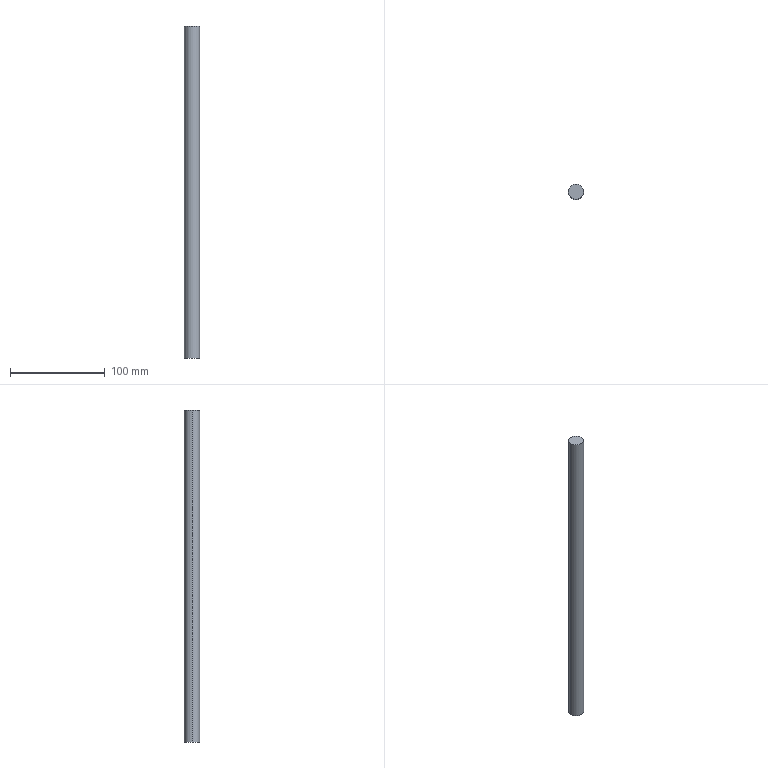Part | SolidWorks | features Extrusion 1 | 1 solid | 4 faces | box 16 x 16 x 350 mm | volume 70372 mm3 | cylinder 2 | plane 2 | commonest cylinder face diameters 16 x2
STEP:
#1=CARTESIAN_POINT('',(8.,0.,350.));
#2=VERTEX_POINT('',#1);
#3=CARTESIAN_POINT('',(-8.,0.,350.));
#4=VERTEX_POINT('',#3);
#5=CARTESIAN_POINT('',(0.,0.,350.));
#6=DIRECTION('',(0.,0.,1.));
#7=DIRECTION('',(1.,0.,0.));
#8=AXIS2_PLACEMENT_3D('',#5,#6,#7);
#9=CIRCLE('',#8,8.);
#10=EDGE_CURVE('',#2,#4,#9,.T.);
#11=ORIENTED_EDGE('',*,*,#10,.F.);
#12=CARTESIAN_POINT('',(8.,0.,0.));
#13=VERTEX_POINT('',#12);
#14=CARTESIAN_POINT('',(8.,0.,350.));
#15=DIRECTION('',(0.,0.,-1.));
#16=VECTOR('',#15,1000.);
#17=LINE('',#14,#16);
#18=EDGE_CURVE('',#2,#13,#17,.T.);
#19=ORIENTED_EDGE('',*,*,#18,.T.);
#20=CARTESIAN_POINT('',(-8.,0.,0.));
#21=VERTEX_POINT('',#20);
#22=CARTESIAN_POINT('',(0.,0.,0.));
#23=DIRECTION('',(0.,0.,1.));
#24=DIRECTION('',(1.,0.,0.));
#25=AXIS2_PLACEMENT_3D('',#22,#23,#24);
#26=CIRCLE('',#25,8.);
#27=EDGE_CURVE('',#13,#21,#26,.T.);
#28=ORIENTED_EDGE('',*,*,#27,.T.);
#29=CARTESIAN_POINT('',(-8.,0.,350.));
#30=DIRECTION('',(0.,0.,-1.));
#31=VECTOR('',#30,1000.);
#32=LINE('',#29,#31);
#33=EDGE_CURVE('',#4,#21,#32,.T.);
#34=ORIENTED_EDGE('',*,*,#33,.F.);
#35=EDGE_LOOP('',(#11,#19,#28,#34));
#36=FACE_OUTER_BOUND('',#35,.T.);
#37=CARTESIAN_POINT('',(0.,0.,350.));
#38=DIRECTION('',(0.,0.,-1.));
#39=DIRECTION('',(-1.,0.,0.));
#40=AXIS2_PLACEMENT_3D('',#37,#38,#39);
#41=CYLINDRICAL_SURFACE('',#40,8.);
#42=ADVANCED_FACE('',(#36),#41,.T.);
#43=ORIENTED_EDGE('',*,*,#18,.F.);
#44=CARTESIAN_POINT('',(0.,0.,350.));
#45=DIRECTION('',(0.,0.,1.));
#46=DIRECTION('',(1.,0.,0.));
#47=AXIS2_PLACEMENT_3D('',#44,#45,#46);
#48=CIRCLE('',#47,8.);
#49=EDGE_CURVE('',#4,#2,#48,.T.);
#50=ORIENTED_EDGE('',*,*,#49,.F.);
#51=ORIENTED_EDGE('',*,*,#33,.T.);
#52=CARTESIAN_POINT('',(0.,0.,0.));
#53=DIRECTION('',(0.,0.,1.));
#54=DIRECTION('',(1.,0.,0.));
#55=AXIS2_PLACEMENT_3D('',#52,#53,#54);
#56=CIRCLE('',#55,8.);
#57=EDGE_CURVE('',#21,#13,#56,.T.);
#58=ORIENTED_EDGE('',*,*,#57,.T.);
#59=EDGE_LOOP('',(#43,#50,#51,#58));
#60=FACE_OUTER_BOUND('',#59,.T.);
#61=CARTESIAN_POINT('',(0.,0.,350.));
#62=DIRECTION('',(0.,0.,-1.));
#63=DIRECTION('',(-1.,0.,0.));
#64=AXIS2_PLACEMENT_3D('',#61,#62,#63);
#65=CYLINDRICAL_SURFACE('',#64,8.);
#66=ADVANCED_FACE('',(#60),#65,.T.);
#67=ORIENTED_EDGE('',*,*,#49,.T.);
#68=ORIENTED_EDGE('',*,*,#10,.T.);
#69=EDGE_LOOP('',(#67,#68));
#70=FACE_OUTER_BOUND('',#69,.T.);
#71=CARTESIAN_POINT('',(0.,0.,350.));
#72=DIRECTION('',(0.,0.,1.));
#73=DIRECTION('',(1.,0.,0.));
#74=AXIS2_PLACEMENT_3D('',#71,#72,#73);
#75=PLANE('',#74);
#76=ADVANCED_FACE('',(#70),#75,.T.);
#77=ORIENTED_EDGE('',*,*,#57,.F.);
#78=ORIENTED_EDGE('',*,*,#27,.F.);
#79=EDGE_LOOP('',(#77,#78));
#80=FACE_OUTER_BOUND('',#79,.T.);
#81=CARTESIAN_POINT('',(0.,0.,0.));
#82=DIRECTION('',(0.,0.,1.));
#83=DIRECTION('',(1.,0.,0.));
#84=AXIS2_PLACEMENT_3D('',#81,#82,#83);
#85=PLANE('',#84);
#86=ADVANCED_FACE('',(#80),#85,.F.);
#87=CLOSED_SHELL('',(#42,#66,#76,#86));
#88=MANIFOLD_SOLID_BREP('',#87);
#89=CARTESIAN_POINT('',(0.,0.,0.));
#90=DIRECTION('',(0.,0.,1.));
#91=DIRECTION('',(1.,0.,0.));
#92=AXIS2_PLACEMENT_3D('',#89,#90,#91);
#93=(LENGTH_UNIT()NAMED_UNIT(*)SI_UNIT(.MILLI.,.METRE.));
#94=UNCERTAINTY_MEASURE_WITH_UNIT(LENGTH_MEASURE(0.00001),#93,'','');
#95=(NAMED_UNIT(*)PLANE_ANGLE_UNIT()SI_UNIT($,.RADIAN.));
#96=(NAMED_UNIT(*)SI_UNIT($,.STERADIAN.)SOLID_ANGLE_UNIT());
#97=(GEOMETRIC_REPRESENTATION_CONTEXT(3)GLOBAL_UNCERTAINTY_ASSIGNED_CONTEXT((#94))GLOBAL_UNIT_ASSIGNED_CONTEXT((#93,#95,#96))REPRESENTATION_CONTEXT('',''));
#98=ADVANCED_BREP_SHAPE_REPRESENTATION('',(#88,#92),#97);